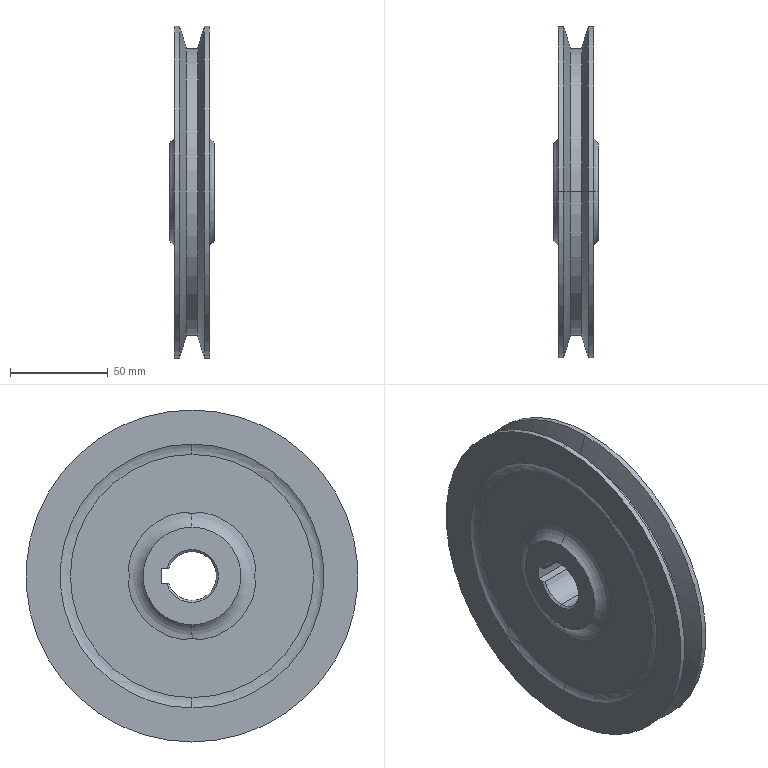Part | SolidWorks | features ICE 4, Cut 2, Chamfer 1, Fillet 1, RevCut 1, Revolution 1 | 1 solid | 46 faces | box 23 x 169.7 x 169.7 mm | volume 320640 mm3 | cylinder 19 | cone 10 | plane 9 | torus 8 | commonest cylinder face diameters 28.4 x10 169.7 x4 25 x3 146.8 x2
STEP:
#1=CARTESIAN_POINT('',(16.5,4.414,-32.703));
#2=VERTEX_POINT('',#1);
#3=CARTESIAN_POINT('',(16.55,0.,-32.));
#4=VERTEX_POINT('',#3);
#5=CARTESIAN_POINT('',(16.5,4.414,-32.703));
#6=CARTESIAN_POINT('',(16.5,3.701,-32.47));
#7=CARTESIAN_POINT('',(16.515,2.977,-32.296));
#8=CARTESIAN_POINT('',(16.534,1.874,-32.119));
#9=CARTESIAN_POINT('',(16.54,1.503,-32.075));
#10=CARTESIAN_POINT('',(16.548,0.7555,-32.015));
#11=CARTESIAN_POINT('',(16.55,0.3773,-32.));
#12=CARTESIAN_POINT('',(16.55,0.,-32.));
#13=B_SPLINE_CURVE_WITH_KNOTS('',3,(#5,#6,#7,#8,#9,#10,#11,#12),.UNSPECIFIED.,.F.,.F.,(4,2,2,4),(0.0008632,0.003097,0.004214,0.00533),.UNSPECIFIED.);
#14=EDGE_CURVE('',#2,#4,#13,.T.);
#15=ORIENTED_EDGE('',*,*,#14,.T.);
#16=CARTESIAN_POINT('',(16.5,0.,-32.));
#17=VERTEX_POINT('',#16);
#18=CARTESIAN_POINT('',(20.5,0.,-32.));
#19=DIRECTION('',(-1.,0.,0.));
#20=VECTOR('',#19,1000.);
#21=LINE('',#18,#20);
#22=EDGE_CURVE('',#4,#17,#21,.T.);
#23=ORIENTED_EDGE('',*,*,#22,.T.);
#24=CARTESIAN_POINT('',(16.5,0.,-46.2));
#25=DIRECTION('',(1.,0.,0.));
#26=DIRECTION('',(0.,0.,-1.));
#27=AXIS2_PLACEMENT_3D('',#24,#25,#26);
#28=CIRCLE('',#27,14.2);
#29=EDGE_CURVE('',#2,#17,#28,.T.);
#30=ORIENTED_EDGE('',*,*,#29,.F.);
#31=EDGE_LOOP('',(#15,#23,#30));
#32=FACE_OUTER_BOUND('',#31,.T.);
#33=CARTESIAN_POINT('',(20.5,0.,-46.2));
#34=DIRECTION('',(-1.,0.,0.));
#35=DIRECTION('',(0.,0.,1.));
#36=AXIS2_PLACEMENT_3D('',#33,#34,#35);
#37=CYLINDRICAL_SURFACE('',#36,14.2);
#38=ADVANCED_FACE('',(#32),#37,.F.);
#39=CARTESIAN_POINT('',(16.5,0.,62.132));
#40=VERTEX_POINT('',#39);
#41=CARTESIAN_POINT('',(16.5,0.,-62.132));
#42=VERTEX_POINT('',#41);
#43=CARTESIAN_POINT('',(16.5,0.,0.));
#44=DIRECTION('',(1.,0.,0.));
#45=DIRECTION('',(0.,0.,1.));
#46=AXIS2_PLACEMENT_3D('',#43,#44,#45);
#47=CIRCLE('',#46,62.132);
#48=EDGE_CURVE('',#40,#42,#47,.T.);
#49=ORIENTED_EDGE('',*,*,#48,.F.);
#50=CARTESIAN_POINT('',(18.,0.,67.4));
#51=VERTEX_POINT('',#50);
#52=CARTESIAN_POINT('',(26.5,0.,62.132));
#53=DIRECTION('',(0.,1.,0.));
#54=DIRECTION('',(0.,0.,1.));
#55=AXIS2_PLACEMENT_3D('',#52,#53,#54);
#56=CIRCLE('',#55,10.);
#57=EDGE_CURVE('',#40,#51,#56,.T.);
#58=ORIENTED_EDGE('',*,*,#57,.T.);
#59=CARTESIAN_POINT('',(18.,0.,-67.4));
#60=VERTEX_POINT('',#59);
#61=CARTESIAN_POINT('',(18.,0.,0.));
#62=DIRECTION('',(-1.,0.,0.));
#63=DIRECTION('',(0.,0.,1.));
#64=AXIS2_PLACEMENT_3D('',#61,#62,#63);
#65=CIRCLE('',#64,67.4);
#66=EDGE_CURVE('',#60,#51,#65,.T.);
#67=ORIENTED_EDGE('',*,*,#66,.F.);
#68=CARTESIAN_POINT('',(26.5,0.,-62.132));
#69=DIRECTION('',(0.,-1.,0.));
#70=DIRECTION('',(0.,0.,-1.));
#71=AXIS2_PLACEMENT_3D('',#68,#69,#70);
#72=CIRCLE('',#71,10.);
#73=EDGE_CURVE('',#42,#60,#72,.T.);
#74=ORIENTED_EDGE('',*,*,#73,.F.);
#75=EDGE_LOOP('',(#49,#58,#67,#74));
#76=FACE_OUTER_BOUND('',#75,.T.);
#77=CARTESIAN_POINT('',(26.5,0.,0.));
#78=DIRECTION('',(1.,0.,0.));
#79=DIRECTION('',(0.,0.,-1.));
#80=AXIS2_PLACEMENT_3D('',#77,#78,#79);
#81=TOROIDAL_SURFACE('',#80,62.132,10.);
#82=ADVANCED_FACE('',(#76),#81,.F.);
#83=CARTESIAN_POINT('',(1.5,0.,-62.132));
#84=VERTEX_POINT('',#83);
#85=CARTESIAN_POINT('',(1.5,0.,62.132));
#86=VERTEX_POINT('',#85);
#87=CARTESIAN_POINT('',(1.5,0.,0.));
#88=DIRECTION('',(-1.,0.,0.));
#89=DIRECTION('',(0.,0.,-1.));
#90=AXIS2_PLACEMENT_3D('',#87,#88,#89);
#91=CIRCLE('',#90,62.132);
#92=EDGE_CURVE('',#84,#86,#91,.T.);
#93=ORIENTED_EDGE('',*,*,#92,.F.);
#94=CARTESIAN_POINT('',(0.,0.,-67.4));
#95=VERTEX_POINT('',#94);
#96=CARTESIAN_POINT('',(-8.5,0.,-62.132));
#97=DIRECTION('',(0.,1.,0.));
#98=DIRECTION('',(0.,0.,1.));
#99=AXIS2_PLACEMENT_3D('',#96,#97,#98);
#100=CIRCLE('',#99,10.);
#101=EDGE_CURVE('',#84,#95,#100,.T.);
#102=ORIENTED_EDGE('',*,*,#101,.T.);
#103=CARTESIAN_POINT('',(0.,0.,67.4));
#104=VERTEX_POINT('',#103);
#105=CARTESIAN_POINT('',(0.,0.,0.));
#106=DIRECTION('',(-1.,0.,0.));
#107=DIRECTION('',(0.,0.,1.));
#108=AXIS2_PLACEMENT_3D('',#105,#106,#107);
#109=CIRCLE('',#108,67.4);
#110=EDGE_CURVE('',#95,#104,#109,.T.);
#111=ORIENTED_EDGE('',*,*,#110,.T.);
#112=CARTESIAN_POINT('',(-8.5,0.,62.132));
#113=DIRECTION('',(0.,-1.,0.));
#114=DIRECTION('',(0.,0.,-1.));
#115=AXIS2_PLACEMENT_3D('',#112,#113,#114);
#116=CIRCLE('',#115,10.);
#117=EDGE_CURVE('',#86,#104,#116,.T.);
#118=ORIENTED_EDGE('',*,*,#117,.F.);
#119=EDGE_LOOP('',(#93,#102,#111,#118));
#120=FACE_OUTER_BOUND('',#119,.T.);
#121=CARTESIAN_POINT('',(-8.5,0.,0.));
#122=DIRECTION('',(-1.,0.,0.));
#123=DIRECTION('',(0.,0.,1.));
#124=AXIS2_PLACEMENT_3D('',#121,#122,#123);
#125=TOROIDAL_SURFACE('',#124,62.132,10.);
#126=ADVANCED_FACE('',(#120),#125,.F.);
#127=CARTESIAN_POINT('',(19.5,0.,12.5));
#128=VERTEX_POINT('',#127);
#129=CARTESIAN_POINT('',(19.5,0.,-12.5));
#130=VERTEX_POINT('',#129);
#131=CARTESIAN_POINT('',(19.5,0.,0.));
#132=DIRECTION('',(1.,0.,0.));
#133=DIRECTION('',(0.,0.,1.));
#134=AXIS2_PLACEMENT_3D('',#131,#132,#133);
#135=CIRCLE('',#134,12.5);
#136=EDGE_CURVE('',#128,#130,#135,.T.);
#137=ORIENTED_EDGE('',*,*,#136,.F.);
#138=CARTESIAN_POINT('',(20.5,0.,13.5));
#139=VERTEX_POINT('',#138);
#140=CARTESIAN_POINT('',(20.5,0.,13.5));
#141=DIRECTION('',(0.7071,0.,0.7071));
#142=VECTOR('',#141,1000.);
#143=LINE('',#140,#142);
#144=EDGE_CURVE('',#128,#139,#143,.T.);
#145=ORIENTED_EDGE('',*,*,#144,.T.);
#146=CARTESIAN_POINT('',(20.5,0.,-13.5));
#147=VERTEX_POINT('',#146);
#148=CARTESIAN_POINT('',(20.5,0.,0.));
#149=DIRECTION('',(-1.,0.,0.));
#150=DIRECTION('',(0.,0.,1.));
#151=AXIS2_PLACEMENT_3D('',#148,#149,#150);
#152=CIRCLE('',#151,13.5);
#153=EDGE_CURVE('',#147,#139,#152,.T.);
#154=ORIENTED_EDGE('',*,*,#153,.F.);
#155=CARTESIAN_POINT('',(20.5,0.,-13.5));
#156=DIRECTION('',(0.7071,0.,-0.7071));
#157=VECTOR('',#156,1000.);
#158=LINE('',#155,#157);
#159=EDGE_CURVE('',#130,#147,#158,.T.);
#160=ORIENTED_EDGE('',*,*,#159,.F.);
#161=EDGE_LOOP('',(#137,#145,#154,#160));
#162=FACE_OUTER_BOUND('',#161,.T.);
#163=CARTESIAN_POINT('',(20.5,0.,0.));
#164=DIRECTION('',(1.,0.,0.));
#165=DIRECTION('',(0.,0.,-1.));
#166=AXIS2_PLACEMENT_3D('',#163,#164,#165);
#167=CONICAL_SURFACE('',#166,13.5,0.7854);
#168=ADVANCED_FACE('',(#162),#167,.F.);
#169=CARTESIAN_POINT('',(19.5,11.843,-4.));
#170=VERTEX_POINT('',#169);
#171=CARTESIAN_POINT('',(19.5,0.,0.));
#172=DIRECTION('',(1.,0.,0.));
#173=DIRECTION('',(0.,0.,1.));
#174=AXIS2_PLACEMENT_3D('',#171,#172,#173);
#175=CIRCLE('',#174,12.5);
#176=EDGE_CURVE('',#130,#170,#175,.T.);
#177=ORIENTED_EDGE('',*,*,#176,.F.);
#178=ORIENTED_EDGE('',*,*,#159,.T.);
#179=CARTESIAN_POINT('',(20.5,12.894,-4.));
#180=VERTEX_POINT('',#179);
#181=CARTESIAN_POINT('',(20.5,0.,0.));
#182=DIRECTION('',(-1.,0.,0.));
#183=DIRECTION('',(0.,0.,1.));
#184=AXIS2_PLACEMENT_3D('',#181,#182,#183);
#185=CIRCLE('',#184,13.5);
#186=EDGE_CURVE('',#180,#147,#185,.T.);
#187=ORIENTED_EDGE('',*,*,#186,.F.);
#188=CARTESIAN_POINT('',(19.5,11.843,-4.));
#189=CARTESIAN_POINT('',(19.833,12.194,-4.));
#190=CARTESIAN_POINT('',(20.166,12.544,-4.));
#191=CARTESIAN_POINT('',(20.5,12.894,-4.));
#192=B_SPLINE_CURVE_WITH_KNOTS('',3,(#188,#189,#190,#191),.UNSPECIFIED.,.F.,.F.,(4,4),(0.00346,0.004911),.UNSPECIFIED.);
#193=EDGE_CURVE('',#170,#180,#192,.T.);
#194=ORIENTED_EDGE('',*,*,#193,.F.);
#195=EDGE_LOOP('',(#177,#178,#187,#194));
#196=FACE_OUTER_BOUND('',#195,.T.);
#197=CARTESIAN_POINT('',(20.5,0.,0.));
#198=DIRECTION('',(1.,0.,0.));
#199=DIRECTION('',(0.,0.,-1.));
#200=AXIS2_PLACEMENT_3D('',#197,#198,#199);
#201=CONICAL_SURFACE('',#200,13.5,0.7854);
#202=ADVANCED_FACE('',(#196),#201,.F.);
#203=CARTESIAN_POINT('',(-1.5,0.,-12.5));
#204=VERTEX_POINT('',#203);
#205=CARTESIAN_POINT('',(-1.5,0.,12.5));
#206=VERTEX_POINT('',#205);
#207=CARTESIAN_POINT('',(-1.5,0.,0.));
#208=DIRECTION('',(-1.,0.,0.));
#209=DIRECTION('',(0.,0.,-1.));
#210=AXIS2_PLACEMENT_3D('',#207,#208,#209);
#211=CIRCLE('',#210,12.5);
#212=EDGE_CURVE('',#204,#206,#211,.T.);
#213=ORIENTED_EDGE('',*,*,#212,.F.);
#214=CARTESIAN_POINT('',(-2.5,0.,-13.5));
#215=VERTEX_POINT('',#214);
#216=CARTESIAN_POINT('',(-1.5,0.,-12.5));
#217=DIRECTION('',(-0.7071,0.,-0.7071));
#218=VECTOR('',#217,1000.);
#219=LINE('',#216,#218);
#220=EDGE_CURVE('',#204,#215,#219,.T.);
#221=ORIENTED_EDGE('',*,*,#220,.T.);
#222=CARTESIAN_POINT('',(-2.5,0.,13.5));
#223=VERTEX_POINT('',#222);
#224=CARTESIAN_POINT('',(-2.5,0.,0.));
#225=DIRECTION('',(1.,0.,0.));
#226=DIRECTION('',(0.,0.,-1.));
#227=AXIS2_PLACEMENT_3D('',#224,#225,#226);
#228=CIRCLE('',#227,13.5);
#229=EDGE_CURVE('',#223,#215,#228,.T.);
#230=ORIENTED_EDGE('',*,*,#229,.F.);
#231=CARTESIAN_POINT('',(-1.5,0.,12.5));
#232=DIRECTION('',(-0.7071,0.,0.7071));
#233=VECTOR('',#232,1000.);
#234=LINE('',#231,#233);
#235=EDGE_CURVE('',#206,#223,#234,.T.);
#236=ORIENTED_EDGE('',*,*,#235,.F.);
#237=EDGE_LOOP('',(#213,#221,#230,#236));
#238=FACE_OUTER_BOUND('',#237,.T.);
#239=CARTESIAN_POINT('',(-1.5,0.,0.));
#240=DIRECTION('',(-1.,0.,0.));
#241=DIRECTION('',(0.,0.,1.));
#242=AXIS2_PLACEMENT_3D('',#239,#240,#241);
#243=CONICAL_SURFACE('',#242,12.5,0.7854);
#244=ADVANCED_FACE('',(#238),#243,.F.);
#245=CARTESIAN_POINT('',(-1.5,11.843,4.));
#246=VERTEX_POINT('',#245);
#247=CARTESIAN_POINT('',(-1.5,0.,0.));
#248=DIRECTION('',(-1.,0.,0.));
#249=DIRECTION('',(0.,0.,-1.));
#250=AXIS2_PLACEMENT_3D('',#247,#248,#249);
#251=CIRCLE('',#250,12.5);
#252=EDGE_CURVE('',#206,#246,#251,.T.);
#253=ORIENTED_EDGE('',*,*,#252,.F.);
#254=ORIENTED_EDGE('',*,*,#235,.T.);
#255=CARTESIAN_POINT('',(-2.5,12.894,4.));
#256=VERTEX_POINT('',#255);
#257=CARTESIAN_POINT('',(-2.5,0.,0.));
#258=DIRECTION('',(1.,0.,0.));
#259=DIRECTION('',(0.,0.,-1.));
#260=AXIS2_PLACEMENT_3D('',#257,#258,#259);
#261=CIRCLE('',#260,13.5);
#262=EDGE_CURVE('',#256,#223,#261,.T.);
#263=ORIENTED_EDGE('',*,*,#262,.F.);
#264=CARTESIAN_POINT('',(-1.5,11.843,4.));
#265=CARTESIAN_POINT('',(-1.833,12.194,4.));
#266=CARTESIAN_POINT('',(-2.166,12.544,4.));
#267=CARTESIAN_POINT('',(-2.5,12.894,4.));
#268=B_SPLINE_CURVE_WITH_KNOTS('',3,(#264,#265,#266,#267),.UNSPECIFIED.,.F.,.F.,(4,4),(0.002815,0.004266),.UNSPECIFIED.);
#269=EDGE_CURVE('',#246,#256,#268,.T.);
#270=ORIENTED_EDGE('',*,*,#269,.F.);
#271=EDGE_LOOP('',(#253,#254,#263,#270));
#272=FACE_OUTER_BOUND('',#271,.T.);
#273=CARTESIAN_POINT('',(-1.5,0.,0.));
#274=DIRECTION('',(-1.,0.,0.));
#275=DIRECTION('',(0.,0.,1.));
#276=AXIS2_PLACEMENT_3D('',#273,#274,#275);
#277=CONICAL_SURFACE('',#276,12.5,0.7854);
#278=ADVANCED_FACE('',(#272),#277,.F.);
#279=CARTESIAN_POINT('',(6.16,0.,73.4));
#280=VERTEX_POINT('',#279);
#281=CARTESIAN_POINT('',(6.16,0.,-73.4));
#282=VERTEX_POINT('',#281);
#283=CARTESIAN_POINT('',(6.16,0.,0.));
#284=DIRECTION('',(-1.,0.,0.));
#285=DIRECTION('',(0.,0.,1.));
#286=AXIS2_PLACEMENT_3D('',#283,#284,#285);
#287=CIRCLE('',#286,73.4);
#288=EDGE_CURVE('',#280,#282,#287,.T.);
#289=ORIENTED_EDGE('',*,*,#288,.T.);
#290=CARTESIAN_POINT('',(2.659,0.,-84.85));
#291=VERTEX_POINT('',#290);
#292=CARTESIAN_POINT('',(2.659,0.,-84.85));
#293=DIRECTION('',(-0.2924,0.,-0.9563));
#294=VECTOR('',#293,1000.);
#295=LINE('',#292,#294);
#296=EDGE_CURVE('',#282,#291,#295,.T.);
#297=ORIENTED_EDGE('',*,*,#296,.T.);
#298=CARTESIAN_POINT('',(2.659,0.,84.85));
#299=VERTEX_POINT('',#298);
#300=CARTESIAN_POINT('',(2.659,0.,0.));
#301=DIRECTION('',(-1.,0.,0.));
#302=DIRECTION('',(0.,0.,1.));
#303=AXIS2_PLACEMENT_3D('',#300,#301,#302);
#304=CIRCLE('',#303,84.85);
#305=EDGE_CURVE('',#299,#291,#304,.T.);
#306=ORIENTED_EDGE('',*,*,#305,.F.);
#307=CARTESIAN_POINT('',(2.659,0.,84.85));
#308=DIRECTION('',(-0.2924,0.,0.9563));
#309=VECTOR('',#308,1000.);
#310=LINE('',#307,#309);
#311=EDGE_CURVE('',#280,#299,#310,.T.);
#312=ORIENTED_EDGE('',*,*,#311,.F.);
#313=EDGE_LOOP('',(#289,#297,#306,#312));
#314=FACE_OUTER_BOUND('',#313,.T.);
#315=CARTESIAN_POINT('',(2.659,0.,0.));
#316=DIRECTION('',(-1.,0.,0.));
#317=DIRECTION('',(0.,0.,1.));
#318=AXIS2_PLACEMENT_3D('',#315,#316,#317);
#319=CONICAL_SURFACE('',#318,84.85,1.274);
#320=ADVANCED_FACE('',(#314),#319,.T.);
#321=CARTESIAN_POINT('',(11.84,0.,73.4));
#322=VERTEX_POINT('',#321);
#323=CARTESIAN_POINT('',(11.84,0.,-73.4));
#324=VERTEX_POINT('',#323);
#325=CARTESIAN_POINT('',(11.84,0.,0.));
#326=DIRECTION('',(-1.,0.,0.));
#327=DIRECTION('',(0.,0.,1.));
#328=AXIS2_PLACEMENT_3D('',#325,#326,#327);
#329=CIRCLE('',#328,73.4);
#330=EDGE_CURVE('',#322,#324,#329,.T.);
#331=ORIENTED_EDGE('',*,*,#330,.F.);
#332=CARTESIAN_POINT('',(15.341,0.,84.85));
#333=VERTEX_POINT('',#332);
#334=CARTESIAN_POINT('',(11.84,0.,73.4));
#335=DIRECTION('',(0.2924,0.,0.9563));
#336=VECTOR('',#335,1000.);
#337=LINE('',#334,#336);
#338=EDGE_CURVE('',#322,#333,#337,.T.);
#339=ORIENTED_EDGE('',*,*,#338,.T.);
#340=CARTESIAN_POINT('',(15.341,0.,-84.85));
#341=VERTEX_POINT('',#340);
#342=CARTESIAN_POINT('',(15.341,0.,0.));
#343=DIRECTION('',(-1.,0.,0.));
#344=DIRECTION('',(0.,0.,1.));
#345=AXIS2_PLACEMENT_3D('',#342,#343,#344);
#346=CIRCLE('',#345,84.85);
#347=EDGE_CURVE('',#333,#341,#346,.T.);
#348=ORIENTED_EDGE('',*,*,#347,.T.);
#349=CARTESIAN_POINT('',(11.84,0.,-73.4));
#350=DIRECTION('',(0.2924,0.,-0.9563));
#351=VECTOR('',#350,1000.);
#352=LINE('',#349,#351);
#353=EDGE_CURVE('',#324,#341,#352,.T.);
#354=ORIENTED_EDGE('',*,*,#353,.F.);
#355=EDGE_LOOP('',(#331,#339,#348,#354));
#356=FACE_OUTER_BOUND('',#355,.T.);
#357=CARTESIAN_POINT('',(11.84,0.,0.));
#358=DIRECTION('',(1.,0.,0.));
#359=DIRECTION('',(0.,0.,-1.));
#360=AXIS2_PLACEMENT_3D('',#357,#358,#359);
#361=CONICAL_SURFACE('',#360,73.4,1.274);
#362=ADVANCED_FACE('',(#356),#361,.T.);
#363=ORIENTED_EDGE('',*,*,#330,.T.);
#364=CARTESIAN_POINT('',(0.,0.,-73.4));
#365=DIRECTION('',(-1.,0.,0.));
#366=VECTOR('',#365,1000.);
#367=LINE('',#364,#366);
#368=EDGE_CURVE('',#324,#282,#367,.T.);
#369=ORIENTED_EDGE('',*,*,#368,.T.);
#370=ORIENTED_EDGE('',*,*,#288,.F.);
#371=CARTESIAN_POINT('',(0.,0.,73.4));
#372=DIRECTION('',(-1.,0.,0.));
#373=VECTOR('',#372,1000.);
#374=LINE('',#371,#373);
#375=EDGE_CURVE('',#322,#280,#374,.T.);
#376=ORIENTED_EDGE('',*,*,#375,.F.);
#377=EDGE_LOOP('',(#363,#369,#370,#376));
#378=FACE_OUTER_BOUND('',#377,.T.);
#379=CARTESIAN_POINT('',(0.,0.,0.));
#380=DIRECTION('',(-1.,0.,0.));
#381=DIRECTION('',(0.,0.,1.));
#382=AXIS2_PLACEMENT_3D('',#379,#380,#381);
#383=CYLINDRICAL_SURFACE('',#382,73.4);
#384=ADVANCED_FACE('',(#378),#383,.T.);
#385=ORIENTED_EDGE('',*,*,#136,.T.);
#386=CARTESIAN_POINT('',(0.,0.,-12.5));
#387=DIRECTION('',(-1.,0.,0.));
#388=VECTOR('',#387,1000.);
#389=LINE('',#386,#388);
#390=EDGE_CURVE('',#130,#204,#389,.T.);
#391=ORIENTED_EDGE('',*,*,#390,.T.);
#392=ORIENTED_EDGE('',*,*,#212,.T.);
#393=CARTESIAN_POINT('',(0.,0.,12.5));
#394=DIRECTION('',(-1.,0.,0.));
#395=VECTOR('',#394,1000.);
#396=LINE('',#393,#395);
#397=EDGE_CURVE('',#128,#206,#396,.T.);
#398=ORIENTED_EDGE('',*,*,#397,.F.);
#399=EDGE_LOOP('',(#385,#391,#392,#398));
#400=FACE_OUTER_BOUND('',#399,.T.);
#401=CARTESIAN_POINT('',(0.,0.,0.));
#402=DIRECTION('',(-1.,0.,0.));
#403=DIRECTION('',(0.,0.,1.));
#404=AXIS2_PLACEMENT_3D('',#401,#402,#403);
#405=CYLINDRICAL_SURFACE('',#404,12.5);
#406=ADVANCED_FACE('',(#400),#405,.F.);
#407=CARTESIAN_POINT('',(19.5,11.843,4.));
#408=VERTEX_POINT('',#407);
#409=CARTESIAN_POINT('',(19.5,0.,0.));
#410=DIRECTION('',(1.,0.,0.));
#411=DIRECTION('',(0.,0.,1.));
#412=AXIS2_PLACEMENT_3D('',#409,#410,#411);
#413=CIRCLE('',#412,12.5);
#414=EDGE_CURVE('',#408,#128,#413,.T.);
#415=ORIENTED_EDGE('',*,*,#414,.T.);
#416=ORIENTED_EDGE('',*,*,#397,.T.);
#417=ORIENTED_EDGE('',*,*,#252,.T.);
#418=CARTESIAN_POINT('',(20.5,11.843,4.));
#419=DIRECTION('',(-1.,0.,0.));
#420=VECTOR('',#419,1000.);
#421=LINE('',#418,#420);
#422=EDGE_CURVE('',#408,#246,#421,.T.);
#423=ORIENTED_EDGE('',*,*,#422,.F.);
#424=EDGE_LOOP('',(#415,#416,#417,#423));
#425=FACE_OUTER_BOUND('',#424,.T.);
#426=CARTESIAN_POINT('',(0.,0.,0.));
#427=DIRECTION('',(-1.,0.,0.));
#428=DIRECTION('',(0.,0.,1.));
#429=AXIS2_PLACEMENT_3D('',#426,#427,#428);
#430=CYLINDRICAL_SURFACE('',#429,12.5);
#431=ADVANCED_FACE('',(#425),#430,.F.);
#432=ORIENTED_EDGE('',*,*,#305,.T.);
#433=CARTESIAN_POINT('',(0.,0.,-84.85));
#434=VERTEX_POINT('',#433);
#435=CARTESIAN_POINT('',(0.,0.,-84.85));
#436=DIRECTION('',(-1.,0.,0.));
#437=VECTOR('',#436,1000.);
#438=LINE('',#435,#437);
#439=EDGE_CURVE('',#291,#434,#438,.T.);
#440=ORIENTED_EDGE('',*,*,#439,.T.);
#441=CARTESIAN_POINT('',(0.,0.,84.85));
#442=VERTEX_POINT('',#441);
#443=CARTESIAN_POINT('',(0.,0.,0.));
#444=DIRECTION('',(-1.,0.,0.));
#445=DIRECTION('',(0.,0.,1.));
#446=AXIS2_PLACEMENT_3D('',#443,#444,#445);
#447=CIRCLE('',#446,84.85);
#448=EDGE_CURVE('',#442,#434,#447,.T.);
#449=ORIENTED_EDGE('',*,*,#448,.F.);
#450=CARTESIAN_POINT('',(0.,0.,84.85));
#451=DIRECTION('',(-1.,0.,0.));
#452=VECTOR('',#451,1000.);
#453=LINE('',#450,#452);
#454=EDGE_CURVE('',#299,#442,#453,.T.);
#455=ORIENTED_EDGE('',*,*,#454,.F.);
#456=EDGE_LOOP('',(#432,#440,#449,#455));
#457=FACE_OUTER_BOUND('',#456,.T.);
#458=CARTESIAN_POINT('',(0.,0.,0.));
#459=DIRECTION('',(-1.,0.,0.));
#460=DIRECTION('',(0.,0.,1.));
#461=AXIS2_PLACEMENT_3D('',#458,#459,#460);
#462=CYLINDRICAL_SURFACE('',#461,84.85);
#463=ADVANCED_FACE('',(#457),#462,.T.);
#464=CARTESIAN_POINT('',(18.,0.,84.85));
#465=VERTEX_POINT('',#464);
#466=CARTESIAN_POINT('',(18.,0.,-84.85));
#467=VERTEX_POINT('',#466);
#468=CARTESIAN_POINT('',(18.,0.,0.));
#469=DIRECTION('',(-1.,0.,0.));
#470=DIRECTION('',(0.,0.,1.));
#471=AXIS2_PLACEMENT_3D('',#468,#469,#470);
#472=CIRCLE('',#471,84.85);
#473=EDGE_CURVE('',#465,#467,#472,.T.);
#474=ORIENTED_EDGE('',*,*,#473,.T.);
#475=CARTESIAN_POINT('',(0.,0.,-84.85));
#476=DIRECTION('',(-1.,0.,0.));
#477=VECTOR('',#476,1000.);
#478=LINE('',#475,#477);
#479=EDGE_CURVE('',#467,#341,#478,.T.);
#480=ORIENTED_EDGE('',*,*,#479,.T.);
#481=ORIENTED_EDGE('',*,*,#347,.F.);
#482=CARTESIAN_POINT('',(0.,0.,84.85));
#483=DIRECTION('',(-1.,0.,0.));
#484=VECTOR('',#483,1000.);
#485=LINE('',#482,#484);
#486=EDGE_CURVE('',#465,#333,#485,.T.);
#487=ORIENTED_EDGE('',*,*,#486,.F.);
#488=EDGE_LOOP('',(#474,#480,#481,#487));
#489=FACE_OUTER_BOUND('',#488,.T.);
#490=CARTESIAN_POINT('',(0.,0.,0.));
#491=DIRECTION('',(-1.,0.,0.));
#492=DIRECTION('',(0.,0.,1.));
#493=AXIS2_PLACEMENT_3D('',#490,#491,#492);
#494=CYLINDRICAL_SURFACE('',#493,84.85);
#495=ADVANCED_FACE('',(#489),#494,.T.);
#496=CARTESIAN_POINT('',(16.5,-4.414,-32.703));
#497=VERTEX_POINT('',#496);
#498=CARTESIAN_POINT('',(16.55,0.,-32.));
#499=CARTESIAN_POINT('',(16.55,-0.7535,-32.));
#500=CARTESIAN_POINT('',(16.54,-1.498,-32.06));
#501=CARTESIAN_POINT('',(16.515,-2.969,-32.294));
#502=CARTESIAN_POINT('',(16.5,-3.696,-32.469));
#503=CARTESIAN_POINT('',(16.5,-4.414,-32.703));
#504=B_SPLINE_CURVE_WITH_KNOTS('',3,(#498,#499,#500,#501,#502,#503),.UNSPECIFIED.,.F.,.F.,(4,2,4),(0.00533,0.007561,0.009791),.UNSPECIFIED.);
#505=EDGE_CURVE('',#4,#497,#504,.T.);
#506=ORIENTED_EDGE('',*,*,#505,.F.);
#507=CARTESIAN_POINT('',(20.5,0.,-25.));
#508=VERTEX_POINT('',#507);
#509=CARTESIAN_POINT('',(26.5,0.,-33.));
#510=DIRECTION('',(0.,1.,0.));
#511=DIRECTION('',(0.,0.,1.));
#512=AXIS2_PLACEMENT_3D('',#509,#510,#511);
#513=CIRCLE('',#512,10.);
#514=EDGE_CURVE('',#4,#508,#513,.T.);
#515=ORIENTED_EDGE('',*,*,#514,.T.);
#516=CARTESIAN_POINT('',(20.5,0.,25.));
#517=VERTEX_POINT('',#516);
#518=CARTESIAN_POINT('',(20.5,0.,0.));
#519=DIRECTION('',(-1.,0.,0.));
#520=DIRECTION('',(0.,0.,1.));
#521=AXIS2_PLACEMENT_3D('',#518,#519,#520);
#522=CIRCLE('',#521,25.);
#523=EDGE_CURVE('',#508,#517,#522,.T.);
#524=ORIENTED_EDGE('',*,*,#523,.T.);
#525=CARTESIAN_POINT('',(16.55,0.,32.));
#526=VERTEX_POINT('',#525);
#527=CARTESIAN_POINT('',(26.5,0.,33.));
#528=DIRECTION('',(0.,-1.,0.));
#529=DIRECTION('',(0.,0.,-1.));
#530=AXIS2_PLACEMENT_3D('',#527,#528,#529);
#531=CIRCLE('',#530,10.);
#532=EDGE_CURVE('',#526,#517,#531,.T.);
#533=ORIENTED_EDGE('',*,*,#532,.F.);
#534=CARTESIAN_POINT('',(16.5,-4.414,32.703));
#535=VERTEX_POINT('',#534);
#536=CARTESIAN_POINT('',(16.5,-4.414,32.703));
#537=CARTESIAN_POINT('',(16.5,-3.701,32.47));
#538=CARTESIAN_POINT('',(16.515,-2.977,32.296));
#539=CARTESIAN_POINT('',(16.534,-1.874,32.119));
#540=CARTESIAN_POINT('',(16.54,-1.503,32.075));
#541=CARTESIAN_POINT('',(16.548,-0.7555,32.015));
#542=CARTESIAN_POINT('',(16.55,-0.3773,32.));
#543=CARTESIAN_POINT('',(16.55,0.,32.));
#544=B_SPLINE_CURVE_WITH_KNOTS('',3,(#536,#537,#538,#539,#540,#541,#542,#543),.UNSPECIFIED.,.F.,.F.,(4,2,2,4),(0.0008632,0.003097,0.004214,0.00533),.UNSPECIFIED.);
#545=EDGE_CURVE('',#535,#526,#544,.T.);
#546=ORIENTED_EDGE('',*,*,#545,.F.);
#547=CARTESIAN_POINT('',(16.5,-32.703,4.414));
#548=VERTEX_POINT('',#547);
#549=CARTESIAN_POINT('',(16.5,0.,0.));
#550=DIRECTION('',(-1.,0.,0.));
#551=DIRECTION('',(0.,0.,1.));
#552=AXIS2_PLACEMENT_3D('',#549,#550,#551);
#553=CIRCLE('',#552,33.);
#554=EDGE_CURVE('',#548,#535,#553,.T.);
#555=ORIENTED_EDGE('',*,*,#554,.F.);
#556=CARTESIAN_POINT('',(16.5,-32.703,-4.414));
#557=VERTEX_POINT('',#556);
#558=CARTESIAN_POINT('',(16.5,-32.703,-4.414));
#559=CARTESIAN_POINT('',(16.5,-32.471,-3.702));
#560=CARTESIAN_POINT('',(16.515,-32.296,-2.978));
#561=CARTESIAN_POINT('',(16.534,-32.119,-1.876));
#562=CARTESIAN_POINT('',(16.54,-32.075,-1.505));
#563=CARTESIAN_POINT('',(16.548,-32.015,-0.7584));
#564=CARTESIAN_POINT('',(16.55,-32.,-0.3805));
#565=CARTESIAN_POINT('',(16.55,-32.,0.7506));
#566=CARTESIAN_POINT('',(16.54,-32.059,1.496));
#567=CARTESIAN_POINT('',(16.515,-32.294,2.968));
#568=CARTESIAN_POINT('',(16.5,-32.468,3.695));
#569=CARTESIAN_POINT('',(16.5,-32.703,4.414));
#570=B_SPLINE_CURVE_WITH_KNOTS('',3,(#558,#559,#560,#561,#562,#563,#564,#565,#566,#567,#568,#569),.UNSPECIFIED.,.F.,.F.,(4,2,2,2,2,4),(0.0008632,0.003095,0.004211,0.005327,0.007559,0.009791),.UNSPECIFIED.);
#571=EDGE_CURVE('',#557,#548,#570,.T.);
#572=ORIENTED_EDGE('',*,*,#571,.F.);
#573=CARTESIAN_POINT('',(16.5,0.,0.));
#574=DIRECTION('',(-1.,0.,0.));
#575=DIRECTION('',(0.,0.,1.));
#576=AXIS2_PLACEMENT_3D('',#573,#574,#575);
#577=CIRCLE('',#576,33.);
#578=EDGE_CURVE('',#497,#557,#577,.T.);
#579=ORIENTED_EDGE('',*,*,#578,.F.);
#580=EDGE_LOOP('',(#506,#515,#524,#533,#546,#555,#572,#579));
#581=FACE_OUTER_BOUND('',#580,.T.);
#582=CARTESIAN_POINT('',(26.5,0.,0.));
#583=DIRECTION('',(-1.,0.,0.));
#584=DIRECTION('',(0.,0.,1.));
#585=AXIS2_PLACEMENT_3D('',#582,#583,#584);
#586=TOROIDAL_SURFACE('',#585,33.,10.);
#587=ADVANCED_FACE('',(#581),#586,.F.);
#588=CARTESIAN_POINT('',(1.45,0.,32.));
#589=VERTEX_POINT('',#588);
#590=CARTESIAN_POINT('',(1.5,-4.414,32.703));
#591=VERTEX_POINT('',#590);
#592=CARTESIAN_POINT('',(1.45,0.,32.));
#593=CARTESIAN_POINT('',(1.45,-0.7535,32.));
#594=CARTESIAN_POINT('',(1.46,-1.498,32.06));
#595=CARTESIAN_POINT('',(1.485,-2.969,32.294));
#596=CARTESIAN_POINT('',(1.5,-3.696,32.469));
#597=CARTESIAN_POINT('',(1.5,-4.414,32.703));
#598=B_SPLINE_CURVE_WITH_KNOTS('',3,(#592,#593,#594,#595,#596,#597),.UNSPECIFIED.,.F.,.F.,(4,2,4),(0.00533,0.007561,0.009791),.UNSPECIFIED.);
#599=EDGE_CURVE('',#589,#591,#598,.T.);
#600=ORIENTED_EDGE('',*,*,#599,.F.);
#601=CARTESIAN_POINT('',(-2.5,0.,25.));
#602=VERTEX_POINT('',#601);
#603=CARTESIAN_POINT('',(-8.5,0.,33.));
#604=DIRECTION('',(0.,1.,0.));
#605=DIRECTION('',(0.,0.,1.));
#606=AXIS2_PLACEMENT_3D('',#603,#604,#605);
#607=CIRCLE('',#606,10.);
#608=EDGE_CURVE('',#589,#602,#607,.T.);
#609=ORIENTED_EDGE('',*,*,#608,.T.);
#610=CARTESIAN_POINT('',(-2.5,0.,-25.));
#611=VERTEX_POINT('',#610);
#612=CARTESIAN_POINT('',(-2.5,0.,0.));
#613=DIRECTION('',(-1.,0.,0.));
#614=DIRECTION('',(0.,0.,1.));
#615=AXIS2_PLACEMENT_3D('',#612,#613,#614);
#616=CIRCLE('',#615,25.);
#617=EDGE_CURVE('',#611,#602,#616,.T.);
#618=ORIENTED_EDGE('',*,*,#617,.F.);
#619=CARTESIAN_POINT('',(1.45,0.,-32.));
#620=VERTEX_POINT('',#619);
#621=CARTESIAN_POINT('',(-8.5,0.,-33.));
#622=DIRECTION('',(0.,-1.,0.));
#623=DIRECTION('',(0.,0.,-1.));
#624=AXIS2_PLACEMENT_3D('',#621,#622,#623);
#625=CIRCLE('',#624,10.);
#626=EDGE_CURVE('',#620,#611,#625,.T.);
#627=ORIENTED_EDGE('',*,*,#626,.F.);
#628=CARTESIAN_POINT('',(1.5,-4.414,-32.703));
#629=VERTEX_POINT('',#628);
#630=CARTESIAN_POINT('',(1.5,-4.414,-32.703));
#631=CARTESIAN_POINT('',(1.5,-3.701,-32.47));
#632=CARTESIAN_POINT('',(1.485,-2.977,-32.296));
#633=CARTESIAN_POINT('',(1.466,-1.874,-32.119));
#634=CARTESIAN_POINT('',(1.46,-1.503,-32.075));
#635=CARTESIAN_POINT('',(1.452,-0.7555,-32.015));
#636=CARTESIAN_POINT('',(1.45,-0.3773,-32.));
#637=CARTESIAN_POINT('',(1.45,0.,-32.));
#638=B_SPLINE_CURVE_WITH_KNOTS('',3,(#630,#631,#632,#633,#634,#635,#636,#637),.UNSPECIFIED.,.F.,.F.,(4,2,2,4),(0.0008632,0.003097,0.004214,0.00533),.UNSPECIFIED.);
#639=EDGE_CURVE('',#629,#620,#638,.T.);
#640=ORIENTED_EDGE('',*,*,#639,.F.);
#641=CARTESIAN_POINT('',(1.5,-32.703,-4.414));
#642=VERTEX_POINT('',#641);
#643=CARTESIAN_POINT('',(1.5,0.,0.));
#644=DIRECTION('',(1.,0.,0.));
#645=DIRECTION('',(0.,0.,-1.));
#646=AXIS2_PLACEMENT_3D('',#643,#644,#645);
#647=CIRCLE('',#646,33.);
#648=EDGE_CURVE('',#642,#629,#647,.T.);
#649=ORIENTED_EDGE('',*,*,#648,.F.);
#650=CARTESIAN_POINT('',(1.5,-32.703,4.414));
#651=VERTEX_POINT('',#650);
#652=CARTESIAN_POINT('',(1.5,-32.703,4.414));
#653=CARTESIAN_POINT('',(1.5,-32.471,3.702));
#654=CARTESIAN_POINT('',(1.485,-32.296,2.978));
#655=CARTESIAN_POINT('',(1.466,-32.119,1.876));
#656=CARTESIAN_POINT('',(1.46,-32.075,1.505));
#657=CARTESIAN_POINT('',(1.452,-32.015,0.7584));
#658=CARTESIAN_POINT('',(1.45,-32.,0.3805));
#659=CARTESIAN_POINT('',(1.45,-32.,-0.7506));
#660=CARTESIAN_POINT('',(1.46,-32.059,-1.496));
#661=CARTESIAN_POINT('',(1.485,-32.294,-2.968));
#662=CARTESIAN_POINT('',(1.5,-32.468,-3.695));
#663=CARTESIAN_POINT('',(1.5,-32.703,-4.414));
#664=B_SPLINE_CURVE_WITH_KNOTS('',3,(#652,#653,#654,#655,#656,#657,#658,#659,#660,#661,#662,#663),.UNSPECIFIED.,.F.,.F.,(4,2,2,2,2,4),(0.0008632,0.003095,0.004211,0.005327,0.007559,0.009791),.UNSPECIFIED.);
#665=EDGE_CURVE('',#651,#642,#664,.T.);
#666=ORIENTED_EDGE('',*,*,#665,.F.);
#667=CARTESIAN_POINT('',(1.5,0.,0.));
#668=DIRECTION('',(1.,0.,0.));
#669=DIRECTION('',(0.,0.,-1.));
#670=AXIS2_PLACEMENT_3D('',#667,#668,#669);
#671=CIRCLE('',#670,33.);
#672=EDGE_CURVE('',#591,#651,#671,.T.);
#673=ORIENTED_EDGE('',*,*,#672,.F.);
#674=EDGE_LOOP('',(#600,#609,#618,#627,#640,#649,#666,#673));
#675=FACE_OUTER_BOUND('',#674,.T.);
#676=CARTESIAN_POINT('',(-8.5,0.,0.));
#677=DIRECTION('',(1.,0.,0.));
#678=DIRECTION('',(0.,0.,-1.));
#679=AXIS2_PLACEMENT_3D('',#676,#677,#678);
#680=TOROIDAL_SURFACE('',#679,33.,10.);
#681=ADVANCED_FACE('',(#675),#680,.F.);
#682=CARTESIAN_POINT('',(1.5,4.414,-32.703));
#683=VERTEX_POINT('',#682);
#684=CARTESIAN_POINT('',(1.5,0.,-32.));
#685=VERTEX_POINT('',#684);
#686=CARTESIAN_POINT('',(1.5,0.,-46.2));
#687=DIRECTION('',(1.,0.,0.));
#688=DIRECTION('',(0.,0.,-1.));
#689=AXIS2_PLACEMENT_3D('',#686,#687,#688);
#690=CIRCLE('',#689,14.2);
#691=EDGE_CURVE('',#683,#685,#690,.T.);
#692=ORIENTED_EDGE('',*,*,#691,.T.);
#693=CARTESIAN_POINT('',(20.5,0.,-32.));
#694=DIRECTION('',(-1.,0.,0.));
#695=VECTOR('',#694,1000.);
#696=LINE('',#693,#695);
#697=EDGE_CURVE('',#685,#620,#696,.T.);
#698=ORIENTED_EDGE('',*,*,#697,.T.);
#699=CARTESIAN_POINT('',(1.45,0.,-32.));
#700=CARTESIAN_POINT('',(1.45,0.7535,-32.));
#701=CARTESIAN_POINT('',(1.46,1.498,-32.06));
#702=CARTESIAN_POINT('',(1.485,2.969,-32.294));
#703=CARTESIAN_POINT('',(1.5,3.696,-32.469));
#704=CARTESIAN_POINT('',(1.5,4.414,-32.703));
#705=B_SPLINE_CURVE_WITH_KNOTS('',3,(#699,#700,#701,#702,#703,#704),.UNSPECIFIED.,.F.,.F.,(4,2,4),(0.00533,0.007561,0.009791),.UNSPECIFIED.);
#706=EDGE_CURVE('',#620,#683,#705,.T.);
#707=ORIENTED_EDGE('',*,*,#706,.T.);
#708=EDGE_LOOP('',(#692,#698,#707));
#709=FACE_OUTER_BOUND('',#708,.T.);
#710=CARTESIAN_POINT('',(20.5,0.,-46.2));
#711=DIRECTION('',(-1.,0.,0.));
#712=DIRECTION('',(0.,0.,1.));
#713=AXIS2_PLACEMENT_3D('',#710,#711,#712);
#714=CYLINDRICAL_SURFACE('',#713,14.2);
#715=ADVANCED_FACE('',(#709),#714,.F.);
#716=ORIENTED_EDGE('',*,*,#665,.T.);
#717=CARTESIAN_POINT('',(1.5,-46.2,0.));
#718=DIRECTION('',(1.,0.,0.));
#719=DIRECTION('',(0.,0.,-1.));
#720=AXIS2_PLACEMENT_3D('',#717,#718,#719);
#721=CIRCLE('',#720,14.2);
#722=EDGE_CURVE('',#642,#651,#721,.T.);
#723=ORIENTED_EDGE('',*,*,#722,.T.);
#724=EDGE_LOOP('',(#716,#723));
#725=FACE_OUTER_BOUND('',#724,.T.);
#726=CARTESIAN_POINT('',(20.5,-46.2,0.));
#727=DIRECTION('',(-1.,0.,0.));
#728=DIRECTION('',(0.,0.,1.));
#729=AXIS2_PLACEMENT_3D('',#726,#727,#728);
#730=CYLINDRICAL_SURFACE('',#729,14.2);
#731=ADVANCED_FACE('',(#725),#730,.F.);
#732=ORIENTED_EDGE('',*,*,#697,.F.);
#733=CARTESIAN_POINT('',(1.5,0.,-46.2));
#734=DIRECTION('',(1.,0.,0.));
#735=DIRECTION('',(0.,0.,-1.));
#736=AXIS2_PLACEMENT_3D('',#733,#734,#735);
#737=CIRCLE('',#736,14.2);
#738=EDGE_CURVE('',#685,#629,#737,.T.);
#739=ORIENTED_EDGE('',*,*,#738,.T.);
#740=ORIENTED_EDGE('',*,*,#639,.T.);
#741=EDGE_LOOP('',(#732,#739,#740));
#742=FACE_OUTER_BOUND('',#741,.T.);
#743=CARTESIAN_POINT('',(20.5,0.,-46.2));
#744=DIRECTION('',(-1.,0.,0.));
#745=DIRECTION('',(0.,0.,1.));
#746=AXIS2_PLACEMENT_3D('',#743,#744,#745);
#747=CYLINDRICAL_SURFACE('',#746,14.2);
#748=ADVANCED_FACE('',(#742),#747,.F.);
#749=CARTESIAN_POINT('',(1.5,32.703,-4.414));
#750=VERTEX_POINT('',#749);
#751=CARTESIAN_POINT('',(1.5,32.703,4.414));
#752=VERTEX_POINT('',#751);
#753=CARTESIAN_POINT('',(1.5,32.703,-4.414));
#754=CARTESIAN_POINT('',(1.5,32.471,-3.702));
#755=CARTESIAN_POINT('',(1.485,32.296,-2.978));
#756=CARTESIAN_POINT('',(1.466,32.119,-1.876));
#757=CARTESIAN_POINT('',(1.46,32.075,-1.505));
#758=CARTESIAN_POINT('',(1.452,32.015,-0.7584));
#759=CARTESIAN_POINT('',(1.45,32.,-0.3805));
#760=CARTESIAN_POINT('',(1.45,32.,0.7506));
#761=CARTESIAN_POINT('',(1.46,32.059,1.496));
#762=CARTESIAN_POINT('',(1.485,32.294,2.968));
#763=CARTESIAN_POINT('',(1.5,32.468,3.695));
#764=CARTESIAN_POINT('',(1.5,32.703,4.414));
#765=B_SPLINE_CURVE_WITH_KNOTS('',3,(#753,#754,#755,#756,#757,#758,#759,#760,#761,#762,#763,#764),.UNSPECIFIED.,.F.,.F.,(4,2,2,2,2,4),(0.0008632,0.003095,0.004211,0.005327,0.007559,0.009791),.UNSPECIFIED.);
#766=EDGE_CURVE('',#750,#752,#765,.T.);
#767=ORIENTED_EDGE('',*,*,#766,.T.);
#768=CARTESIAN_POINT('',(1.5,46.2,0.));
#769=DIRECTION('',(1.,0.,0.));
#770=DIRECTION('',(0.,0.,-1.));
#771=AXIS2_PLACEMENT_3D('',#768,#769,#770);
#772=CIRCLE('',#771,14.2);
#773=EDGE_CURVE('',#752,#750,#772,.T.);
#774=ORIENTED_EDGE('',*,*,#773,.T.);
#775=EDGE_LOOP('',(#767,#774));
#776=FACE_OUTER_BOUND('',#775,.T.);
#777=CARTESIAN_POINT('',(20.5,46.2,0.));
#778=DIRECTION('',(-1.,0.,0.));
#779=DIRECTION('',(0.,0.,1.));
#780=AXIS2_PLACEMENT_3D('',#777,#778,#779);
#781=CYLINDRICAL_SURFACE('',#780,14.2);
#782=ADVANCED_FACE('',(#776),#781,.F.);
#783=CARTESIAN_POINT('',(1.5,4.414,32.703));
#784=VERTEX_POINT('',#783);
#785=CARTESIAN_POINT('',(1.5,4.414,32.703));
#786=CARTESIAN_POINT('',(1.5,3.701,32.47));
#787=CARTESIAN_POINT('',(1.485,2.977,32.296));
#788=CARTESIAN_POINT('',(1.466,1.874,32.119));
#789=CARTESIAN_POINT('',(1.46,1.503,32.075));
#790=CARTESIAN_POINT('',(1.452,0.7555,32.015));
#791=CARTESIAN_POINT('',(1.45,0.3773,32.));
#792=CARTESIAN_POINT('',(1.45,0.,32.));
#793=B_SPLINE_CURVE_WITH_KNOTS('',3,(#785,#786,#787,#788,#789,#790,#791,#792),.UNSPECIFIED.,.F.,.F.,(4,2,2,4),(0.0008632,0.003097,0.004214,0.00533),.UNSPECIFIED.);
#794=EDGE_CURVE('',#784,#589,#793,.T.);
#795=ORIENTED_EDGE('',*,*,#794,.T.);
#796=ORIENTED_EDGE('',*,*,#599,.T.);
#797=CARTESIAN_POINT('',(1.5,0.,46.2));
#798=DIRECTION('',(1.,0.,0.));
#799=DIRECTION('',(0.,0.,-1.));
#800=AXIS2_PLACEMENT_3D('',#797,#798,#799);
#801=CIRCLE('',#800,14.2);
#802=EDGE_CURVE('',#591,#784,#801,.T.);
#803=ORIENTED_EDGE('',*,*,#802,.T.);
#804=EDGE_LOOP('',(#795,#796,#803));
#805=FACE_OUTER_BOUND('',#804,.T.);
#806=CARTESIAN_POINT('',(20.5,0.,46.2));
#807=DIRECTION('',(-1.,0.,0.));
#808=DIRECTION('',(0.,0.,1.));
#809=AXIS2_PLACEMENT_3D('',#806,#807,#808);
#810=CYLINDRICAL_SURFACE('',#809,14.2);
#811=ADVANCED_FACE('',(#805),#810,.F.);
#812=CARTESIAN_POINT('',(1.5,0.,0.));
#813=DIRECTION('',(-1.,0.,0.));
#814=DIRECTION('',(0.,0.,-1.));
#815=AXIS2_PLACEMENT_3D('',#812,#813,#814);
#816=CIRCLE('',#815,62.132);
#817=EDGE_CURVE('',#86,#84,#816,.T.);
#818=ORIENTED_EDGE('',*,*,#817,.T.);
#819=ORIENTED_EDGE('',*,*,#92,.T.);
#820=EDGE_LOOP('',(#818,#819));
#821=FACE_OUTER_BOUND('',#820,.T.);
#822=CARTESIAN_POINT('',(1.5,0.,0.));
#823=DIRECTION('',(1.,0.,0.));
#824=DIRECTION('',(0.,0.,-1.));
#825=AXIS2_PLACEMENT_3D('',#822,#823,#824);
#826=CIRCLE('',#825,33.);
#827=EDGE_CURVE('',#752,#784,#826,.T.);
#828=ORIENTED_EDGE('',*,*,#827,.T.);
#829=ORIENTED_EDGE('',*,*,#802,.F.);
#830=ORIENTED_EDGE('',*,*,#672,.T.);
#831=ORIENTED_EDGE('',*,*,#722,.F.);
#832=ORIENTED_EDGE('',*,*,#648,.T.);
#833=ORIENTED_EDGE('',*,*,#738,.F.);
#834=ORIENTED_EDGE('',*,*,#691,.F.);
#835=CARTESIAN_POINT('',(1.5,0.,0.));
#836=DIRECTION('',(1.,0.,0.));
#837=DIRECTION('',(0.,0.,-1.));
#838=AXIS2_PLACEMENT_3D('',#835,#836,#837);
#839=CIRCLE('',#838,33.);
#840=EDGE_CURVE('',#683,#750,#839,.T.);
#841=ORIENTED_EDGE('',*,*,#840,.T.);
#842=ORIENTED_EDGE('',*,*,#773,.F.);
#843=EDGE_LOOP('',(#828,#829,#830,#831,#832,#833,#834,#841,#842));
#844=FACE_BOUND('',#843,.T.);
#845=CARTESIAN_POINT('',(1.5,25.35,0.));
#846=DIRECTION('',(1.,0.,0.));
#847=DIRECTION('',(0.,0.,-1.));
#848=AXIS2_PLACEMENT_3D('',#845,#846,#847);
#849=PLANE('',#848);
#850=ADVANCED_FACE('',(#821,#844),#849,.F.);
#851=CARTESIAN_POINT('',(16.5,0.,0.));
#852=DIRECTION('',(1.,0.,0.));
#853=DIRECTION('',(0.,0.,1.));
#854=AXIS2_PLACEMENT_3D('',#851,#852,#853);
#855=CIRCLE('',#854,62.132);
#856=EDGE_CURVE('',#42,#40,#855,.T.);
#857=ORIENTED_EDGE('',*,*,#856,.T.);
#858=ORIENTED_EDGE('',*,*,#48,.T.);
#859=EDGE_LOOP('',(#857,#858));
#860=FACE_OUTER_BOUND('',#859,.T.);
#861=ORIENTED_EDGE('',*,*,#554,.T.);
#862=CARTESIAN_POINT('',(16.5,4.414,32.703));
#863=VERTEX_POINT('',#862);
#864=CARTESIAN_POINT('',(16.5,0.,46.2));
#865=DIRECTION('',(1.,0.,0.));
#866=DIRECTION('',(0.,0.,-1.));
#867=AXIS2_PLACEMENT_3D('',#864,#865,#866);
#868=CIRCLE('',#867,14.2);
#869=EDGE_CURVE('',#535,#863,#868,.T.);
#870=ORIENTED_EDGE('',*,*,#869,.T.);
#871=CARTESIAN_POINT('',(16.5,32.703,4.414));
#872=VERTEX_POINT('',#871);
#873=CARTESIAN_POINT('',(16.5,0.,0.));
#874=DIRECTION('',(-1.,0.,0.));
#875=DIRECTION('',(0.,0.,1.));
#876=AXIS2_PLACEMENT_3D('',#873,#874,#875);
#877=CIRCLE('',#876,33.);
#878=EDGE_CURVE('',#863,#872,#877,.T.);
#879=ORIENTED_EDGE('',*,*,#878,.T.);
#880=CARTESIAN_POINT('',(16.5,32.703,-4.414));
#881=VERTEX_POINT('',#880);
#882=CARTESIAN_POINT('',(16.5,46.2,0.));
#883=DIRECTION('',(1.,0.,0.));
#884=DIRECTION('',(0.,0.,-1.));
#885=AXIS2_PLACEMENT_3D('',#882,#883,#884);
#886=CIRCLE('',#885,14.2);
#887=EDGE_CURVE('',#872,#881,#886,.T.);
#888=ORIENTED_EDGE('',*,*,#887,.T.);
#889=CARTESIAN_POINT('',(16.5,0.,0.));
#890=DIRECTION('',(-1.,0.,0.));
#891=DIRECTION('',(0.,0.,1.));
#892=AXIS2_PLACEMENT_3D('',#889,#890,#891);
#893=CIRCLE('',#892,33.);
#894=EDGE_CURVE('',#881,#2,#893,.T.);
#895=ORIENTED_EDGE('',*,*,#894,.T.);
#896=ORIENTED_EDGE('',*,*,#29,.T.);
#897=CARTESIAN_POINT('',(16.5,0.,-46.2));
#898=DIRECTION('',(1.,0.,0.));
#899=DIRECTION('',(0.,0.,-1.));
#900=AXIS2_PLACEMENT_3D('',#897,#898,#899);
#901=CIRCLE('',#900,14.2);
#902=EDGE_CURVE('',#17,#497,#901,.T.);
#903=ORIENTED_EDGE('',*,*,#902,.T.);
#904=ORIENTED_EDGE('',*,*,#578,.T.);
#905=CARTESIAN_POINT('',(16.5,-46.2,0.));
#906=DIRECTION('',(1.,0.,0.));
#907=DIRECTION('',(0.,0.,-1.));
#908=AXIS2_PLACEMENT_3D('',#905,#906,#907);
#909=CIRCLE('',#908,14.2);
#910=EDGE_CURVE('',#557,#548,#909,.T.);
#911=ORIENTED_EDGE('',*,*,#910,.T.);
#912=EDGE_LOOP('',(#861,#870,#879,#888,#895,#896,#903,#904,#911));
#913=FACE_BOUND('',#912,.T.);
#914=CARTESIAN_POINT('',(16.5,67.269,0.));
#915=DIRECTION('',(-1.,0.,0.));
#916=DIRECTION('',(0.,0.,1.));
#917=AXIS2_PLACEMENT_3D('',#914,#915,#916);
#918=PLANE('',#917);
#919=ADVANCED_FACE('',(#860,#913),#918,.F.);
#920=ORIENTED_EDGE('',*,*,#608,.F.);
#921=ORIENTED_EDGE('',*,*,#794,.F.);
#922=ORIENTED_EDGE('',*,*,#827,.F.);
#923=ORIENTED_EDGE('',*,*,#766,.F.);
#924=ORIENTED_EDGE('',*,*,#840,.F.);
#925=ORIENTED_EDGE('',*,*,#706,.F.);
#926=ORIENTED_EDGE('',*,*,#626,.T.);
#927=CARTESIAN_POINT('',(-2.5,0.,0.));
#928=DIRECTION('',(-1.,0.,0.));
#929=DIRECTION('',(0.,0.,1.));
#930=AXIS2_PLACEMENT_3D('',#927,#928,#929);
#931=CIRCLE('',#930,25.);
#932=EDGE_CURVE('',#602,#611,#931,.T.);
#933=ORIENTED_EDGE('',*,*,#932,.F.);
#934=EDGE_LOOP('',(#920,#921,#922,#923,#924,#925,#926,#933));
#935=FACE_OUTER_BOUND('',#934,.T.);
#936=CARTESIAN_POINT('',(-8.5,0.,0.));
#937=DIRECTION('',(1.,0.,0.));
#938=DIRECTION('',(0.,0.,-1.));
#939=AXIS2_PLACEMENT_3D('',#936,#937,#938);
#940=TOROIDAL_SURFACE('',#939,33.,10.);
#941=ADVANCED_FACE('',(#935),#940,.F.);
#942=ORIENTED_EDGE('',*,*,#514,.F.);
#943=ORIENTED_EDGE('',*,*,#14,.F.);
#944=ORIENTED_EDGE('',*,*,#894,.F.);
#945=CARTESIAN_POINT('',(16.5,32.703,4.414));
#946=CARTESIAN_POINT('',(16.5,32.471,3.702));
#947=CARTESIAN_POINT('',(16.515,32.296,2.978));
#948=CARTESIAN_POINT('',(16.534,32.119,1.876));
#949=CARTESIAN_POINT('',(16.54,32.075,1.505));
#950=CARTESIAN_POINT('',(16.548,32.015,0.7584));
#951=CARTESIAN_POINT('',(16.55,32.,0.3805));
#952=CARTESIAN_POINT('',(16.55,32.,-0.7506));
#953=CARTESIAN_POINT('',(16.54,32.059,-1.496));
#954=CARTESIAN_POINT('',(16.515,32.294,-2.968));
#955=CARTESIAN_POINT('',(16.5,32.468,-3.695));
#956=CARTESIAN_POINT('',(16.5,32.703,-4.414));
#957=B_SPLINE_CURVE_WITH_KNOTS('',3,(#945,#946,#947,#948,#949,#950,#951,#952,#953,#954,#955,#956),.UNSPECIFIED.,.F.,.F.,(4,2,2,2,2,4),(0.0008632,0.003095,0.004211,0.005327,0.007559,0.009791),.UNSPECIFIED.);
#958=EDGE_CURVE('',#872,#881,#957,.T.);
#959=ORIENTED_EDGE('',*,*,#958,.F.);
#960=ORIENTED_EDGE('',*,*,#878,.F.);
#961=CARTESIAN_POINT('',(16.55,0.,32.));
#962=CARTESIAN_POINT('',(16.55,0.7535,32.));
#963=CARTESIAN_POINT('',(16.54,1.498,32.06));
#964=CARTESIAN_POINT('',(16.515,2.969,32.294));
#965=CARTESIAN_POINT('',(16.5,3.696,32.469));
#966=CARTESIAN_POINT('',(16.5,4.414,32.703));
#967=B_SPLINE_CURVE_WITH_KNOTS('',3,(#961,#962,#963,#964,#965,#966),.UNSPECIFIED.,.F.,.F.,(4,2,4),(0.00533,0.007561,0.009791),.UNSPECIFIED.);
#968=EDGE_CURVE('',#526,#863,#967,.T.);
#969=ORIENTED_EDGE('',*,*,#968,.F.);
#970=ORIENTED_EDGE('',*,*,#532,.T.);
#971=CARTESIAN_POINT('',(20.5,0.,0.));
#972=DIRECTION('',(-1.,0.,0.));
#973=DIRECTION('',(0.,0.,1.));
#974=AXIS2_PLACEMENT_3D('',#971,#972,#973);
#975=CIRCLE('',#974,25.);
#976=EDGE_CURVE('',#517,#508,#975,.T.);
#977=ORIENTED_EDGE('',*,*,#976,.T.);
#978=EDGE_LOOP('',(#942,#943,#944,#959,#960,#969,#970,#977));
#979=FACE_OUTER_BOUND('',#978,.T.);
#980=CARTESIAN_POINT('',(26.5,0.,0.));
#981=DIRECTION('',(-1.,0.,0.));
#982=DIRECTION('',(0.,0.,1.));
#983=AXIS2_PLACEMENT_3D('',#980,#981,#982);
#984=TOROIDAL_SURFACE('',#983,33.,10.);
#985=ADVANCED_FACE('',(#979),#984,.F.);
#986=ORIENTED_EDGE('',*,*,#479,.F.);
#987=CARTESIAN_POINT('',(18.,0.,0.));
#988=DIRECTION('',(-1.,0.,0.));
#989=DIRECTION('',(0.,0.,1.));
#990=AXIS2_PLACEMENT_3D('',#987,#988,#989);
#991=CIRCLE('',#990,84.85);
#992=EDGE_CURVE('',#467,#465,#991,.T.);
#993=ORIENTED_EDGE('',*,*,#992,.T.);
#994=ORIENTED_EDGE('',*,*,#486,.T.);
#995=CARTESIAN_POINT('',(15.341,0.,0.));
#996=DIRECTION('',(-1.,0.,0.));
#997=DIRECTION('',(0.,0.,1.));
#998=AXIS2_PLACEMENT_3D('',#995,#996,#997);
#999=CIRCLE('',#998,84.85);
#1000=EDGE_CURVE('',#341,#333,#999,.T.);
#1001=ORIENTED_EDGE('',*,*,#1000,.F.);
#1002=EDGE_LOOP('',(#986,#993,#994,#1001));
#1003=FACE_OUTER_BOUND('',#1002,.T.);
#1004=CARTESIAN_POINT('',(0.,0.,0.));
#1005=DIRECTION('',(-1.,0.,0.));
#1006=DIRECTION('',(0.,0.,1.));
#1007=AXIS2_PLACEMENT_3D('',#1004,#1005,#1006);
#1008=CYLINDRICAL_SURFACE('',#1007,84.85);
#1009=ADVANCED_FACE('',(#1003),#1008,.T.);
#1010=ORIENTED_EDGE('',*,*,#439,.F.);
#1011=CARTESIAN_POINT('',(2.659,0.,0.));
#1012=DIRECTION('',(-1.,0.,0.));
#1013=DIRECTION('',(0.,0.,1.));
#1014=AXIS2_PLACEMENT_3D('',#1011,#1012,#1013);
#1015=CIRCLE('',#1014,84.85);
#1016=EDGE_CURVE('',#291,#299,#1015,.T.);
#1017=ORIENTED_EDGE('',*,*,#1016,.T.);
#1018=ORIENTED_EDGE('',*,*,#454,.T.);
#1019=CARTESIAN_POINT('',(0.,0.,0.));
#1020=DIRECTION('',(-1.,0.,0.));
#1021=DIRECTION('',(0.,0.,1.));
#1022=AXIS2_PLACEMENT_3D('',#1019,#1020,#1021);
#1023=CIRCLE('',#1022,84.85);
#1024=EDGE_CURVE('',#434,#442,#1023,.T.);
#1025=ORIENTED_EDGE('',*,*,#1024,.F.);
#1026=EDGE_LOOP('',(#1010,#1017,#1018,#1025));
#1027=FACE_OUTER_BOUND('',#1026,.T.);
#1028=CARTESIAN_POINT('',(0.,0.,0.));
#1029=DIRECTION('',(-1.,0.,0.));
#1030=DIRECTION('',(0.,0.,1.));
#1031=AXIS2_PLACEMENT_3D('',#1028,#1029,#1030);
#1032=CYLINDRICAL_SURFACE('',#1031,84.85);
#1033=ADVANCED_FACE('',(#1027),#1032,.T.);
#1034=ORIENTED_EDGE('',*,*,#390,.F.);
#1035=ORIENTED_EDGE('',*,*,#176,.T.);
#1036=CARTESIAN_POINT('',(-1.5,11.843,-4.));
#1037=VERTEX_POINT('',#1036);
#1038=CARTESIAN_POINT('',(20.5,11.843,-4.));
#1039=DIRECTION('',(-1.,0.,0.));
#1040=VECTOR('',#1039,1000.);
#1041=LINE('',#1038,#1040);
#1042=EDGE_CURVE('',#170,#1037,#1041,.T.);
#1043=ORIENTED_EDGE('',*,*,#1042,.T.);
#1044=CARTESIAN_POINT('',(-1.5,0.,0.));
#1045=DIRECTION('',(-1.,0.,0.));
#1046=DIRECTION('',(0.,0.,-1.));
#1047=AXIS2_PLACEMENT_3D('',#1044,#1045,#1046);
#1048=CIRCLE('',#1047,12.5);
#1049=EDGE_CURVE('',#1037,#204,#1048,.T.);
#1050=ORIENTED_EDGE('',*,*,#1049,.T.);
#1051=EDGE_LOOP('',(#1034,#1035,#1043,#1050));
#1052=FACE_OUTER_BOUND('',#1051,.T.);
#1053=CARTESIAN_POINT('',(0.,0.,0.));
#1054=DIRECTION('',(-1.,0.,0.));
#1055=DIRECTION('',(0.,0.,1.));
#1056=AXIS2_PLACEMENT_3D('',#1053,#1054,#1055);
#1057=CYLINDRICAL_SURFACE('',#1056,12.5);
#1058=ADVANCED_FACE('',(#1052),#1057,.F.);
#1059=ORIENTED_EDGE('',*,*,#262,.T.);
#1060=ORIENTED_EDGE('',*,*,#229,.T.);
#1061=CARTESIAN_POINT('',(-2.5,12.894,-4.));
#1062=VERTEX_POINT('',#1061);
#1063=CARTESIAN_POINT('',(-2.5,0.,0.));
#1064=DIRECTION('',(1.,0.,0.));
#1065=DIRECTION('',(0.,0.,-1.));
#1066=AXIS2_PLACEMENT_3D('',#1063,#1064,#1065);
#1067=CIRCLE('',#1066,13.5);
#1068=EDGE_CURVE('',#215,#1062,#1067,.T.);
#1069=ORIENTED_EDGE('',*,*,#1068,.T.);
#1070=CARTESIAN_POINT('',(-2.5,15.8,-4.));
#1071=VERTEX_POINT('',#1070);
#1072=CARTESIAN_POINT('',(-2.5,11.843,-4.));
#1073=DIRECTION('',(0.,-1.,0.));
#1074=VECTOR('',#1073,1000.);
#1075=LINE('',#1072,#1074);
#1076=EDGE_CURVE('',#1071,#1062,#1075,.T.);
#1077=ORIENTED_EDGE('',*,*,#1076,.F.);
#1078=CARTESIAN_POINT('',(-2.5,15.8,4.));
#1079=VERTEX_POINT('',#1078);
#1080=CARTESIAN_POINT('',(-2.5,15.8,-4.));
#1081=DIRECTION('',(0.,0.,-1.));
#1082=VECTOR('',#1081,1000.);
#1083=LINE('',#1080,#1082);
#1084=EDGE_CURVE('',#1079,#1071,#1083,.T.);
#1085=ORIENTED_EDGE('',*,*,#1084,.F.);
#1086=CARTESIAN_POINT('',(-2.5,11.843,4.));
#1087=DIRECTION('',(0.,1.,0.));
#1088=VECTOR('',#1087,1000.);
#1089=LINE('',#1086,#1088);
#1090=EDGE_CURVE('',#256,#1079,#1089,.T.);
#1091=ORIENTED_EDGE('',*,*,#1090,.F.);
#1092=EDGE_LOOP('',(#1059,#1060,#1069,#1077,#1085,#1091));
#1093=FACE_BOUND('',#1092,.T.);
#1094=ORIENTED_EDGE('',*,*,#617,.T.);
#1095=ORIENTED_EDGE('',*,*,#932,.T.);
#1096=EDGE_LOOP('',(#1094,#1095));
#1097=FACE_OUTER_BOUND('',#1096,.T.);
#1098=CARTESIAN_POINT('',(-2.5,12.5,0.));
#1099=DIRECTION('',(1.,0.,0.));
#1100=DIRECTION('',(0.,0.,-1.));
#1101=AXIS2_PLACEMENT_3D('',#1098,#1099,#1100);
#1102=PLANE('',#1101);
#1103=ADVANCED_FACE('',(#1093,#1097),#1102,.F.);
#1104=CARTESIAN_POINT('',(0.,0.,0.));
#1105=DIRECTION('',(-1.,0.,0.));
#1106=DIRECTION('',(0.,0.,1.));
#1107=AXIS2_PLACEMENT_3D('',#1104,#1105,#1106);
#1108=CIRCLE('',#1107,67.4);
#1109=EDGE_CURVE('',#104,#95,#1108,.T.);
#1110=ORIENTED_EDGE('',*,*,#1109,.F.);
#1111=ORIENTED_EDGE('',*,*,#110,.F.);
#1112=EDGE_LOOP('',(#1110,#1111));
#1113=FACE_BOUND('',#1112,.T.);
#1114=ORIENTED_EDGE('',*,*,#448,.T.);
#1115=ORIENTED_EDGE('',*,*,#1024,.T.);
#1116=EDGE_LOOP('',(#1114,#1115));
#1117=FACE_OUTER_BOUND('',#1116,.T.);
#1118=CARTESIAN_POINT('',(0.,67.4,0.));
#1119=DIRECTION('',(1.,0.,0.));
#1120=DIRECTION('',(0.,0.,-1.));
#1121=AXIS2_PLACEMENT_3D('',#1118,#1119,#1120);
#1122=PLANE('',#1121);
#1123=ADVANCED_FACE('',(#1113,#1117),#1122,.F.);
#1124=ORIENTED_EDGE('',*,*,#473,.F.);
#1125=ORIENTED_EDGE('',*,*,#992,.F.);
#1126=EDGE_LOOP('',(#1124,#1125));
#1127=FACE_OUTER_BOUND('',#1126,.T.);
#1128=ORIENTED_EDGE('',*,*,#66,.T.);
#1129=CARTESIAN_POINT('',(18.,0.,0.));
#1130=DIRECTION('',(-1.,0.,0.));
#1131=DIRECTION('',(0.,0.,1.));
#1132=AXIS2_PLACEMENT_3D('',#1129,#1130,#1131);
#1133=CIRCLE('',#1132,67.4);
#1134=EDGE_CURVE('',#51,#60,#1133,.T.);
#1135=ORIENTED_EDGE('',*,*,#1134,.T.);
#1136=EDGE_LOOP('',(#1128,#1135));
#1137=FACE_BOUND('',#1136,.T.);
#1138=CARTESIAN_POINT('',(18.,84.85,0.));
#1139=DIRECTION('',(-1.,0.,0.));
#1140=DIRECTION('',(0.,0.,1.));
#1141=AXIS2_PLACEMENT_3D('',#1138,#1139,#1140);
#1142=PLANE('',#1141);
#1143=ADVANCED_FACE('',(#1127,#1137),#1142,.F.);
#1144=CARTESIAN_POINT('',(20.5,15.8,4.));
#1145=VERTEX_POINT('',#1144);
#1146=CARTESIAN_POINT('',(20.5,15.8,-4.));
#1147=VERTEX_POINT('',#1146);
#1148=CARTESIAN_POINT('',(20.5,15.8,-4.));
#1149=DIRECTION('',(0.,0.,-1.));
#1150=VECTOR('',#1149,1000.);
#1151=LINE('',#1148,#1150);
#1152=EDGE_CURVE('',#1145,#1147,#1151,.T.);
#1153=ORIENTED_EDGE('',*,*,#1152,.T.);
#1154=CARTESIAN_POINT('',(20.5,11.843,-4.));
#1155=DIRECTION('',(0.,-1.,0.));
#1156=VECTOR('',#1155,1000.);
#1157=LINE('',#1154,#1156);
#1158=EDGE_CURVE('',#1147,#180,#1157,.T.);
#1159=ORIENTED_EDGE('',*,*,#1158,.T.);
#1160=ORIENTED_EDGE('',*,*,#186,.T.);
#1161=ORIENTED_EDGE('',*,*,#153,.T.);
#1162=CARTESIAN_POINT('',(20.5,12.894,4.));
#1163=VERTEX_POINT('',#1162);
#1164=CARTESIAN_POINT('',(20.5,0.,0.));
#1165=DIRECTION('',(-1.,0.,0.));
#1166=DIRECTION('',(0.,0.,1.));
#1167=AXIS2_PLACEMENT_3D('',#1164,#1165,#1166);
#1168=CIRCLE('',#1167,13.5);
#1169=EDGE_CURVE('',#139,#1163,#1168,.T.);
#1170=ORIENTED_EDGE('',*,*,#1169,.T.);
#1171=CARTESIAN_POINT('',(20.5,11.843,4.));
#1172=DIRECTION('',(0.,1.,0.));
#1173=VECTOR('',#1172,1000.);
#1174=LINE('',#1171,#1173);
#1175=EDGE_CURVE('',#1163,#1145,#1174,.T.);
#1176=ORIENTED_EDGE('',*,*,#1175,.T.);
#1177=EDGE_LOOP('',(#1153,#1159,#1160,#1161,#1170,#1176));
#1178=FACE_BOUND('',#1177,.T.);
#1179=ORIENTED_EDGE('',*,*,#976,.F.);
#1180=ORIENTED_EDGE('',*,*,#523,.F.);
#1181=EDGE_LOOP('',(#1179,#1180));
#1182=FACE_OUTER_BOUND('',#1181,.T.);
#1183=CARTESIAN_POINT('',(20.5,25.,0.));
#1184=DIRECTION('',(-1.,0.,0.));
#1185=DIRECTION('',(0.,0.,1.));
#1186=AXIS2_PLACEMENT_3D('',#1183,#1184,#1185);
#1187=PLANE('',#1186);
#1188=ADVANCED_FACE('',(#1178,#1182),#1187,.F.);
#1189=ORIENTED_EDGE('',*,*,#368,.F.);
#1190=CARTESIAN_POINT('',(11.84,0.,0.));
#1191=DIRECTION('',(-1.,0.,0.));
#1192=DIRECTION('',(0.,0.,1.));
#1193=AXIS2_PLACEMENT_3D('',#1190,#1191,#1192);
#1194=CIRCLE('',#1193,73.4);
#1195=EDGE_CURVE('',#324,#322,#1194,.T.);
#1196=ORIENTED_EDGE('',*,*,#1195,.T.);
#1197=ORIENTED_EDGE('',*,*,#375,.T.);
#1198=CARTESIAN_POINT('',(6.16,0.,0.));
#1199=DIRECTION('',(-1.,0.,0.));
#1200=DIRECTION('',(0.,0.,1.));
#1201=AXIS2_PLACEMENT_3D('',#1198,#1199,#1200);
#1202=CIRCLE('',#1201,73.4);
#1203=EDGE_CURVE('',#282,#280,#1202,.T.);
#1204=ORIENTED_EDGE('',*,*,#1203,.F.);
#1205=EDGE_LOOP('',(#1189,#1196,#1197,#1204));
#1206=FACE_OUTER_BOUND('',#1205,.T.);
#1207=CARTESIAN_POINT('',(0.,0.,0.));
#1208=DIRECTION('',(-1.,0.,0.));
#1209=DIRECTION('',(0.,0.,1.));
#1210=AXIS2_PLACEMENT_3D('',#1207,#1208,#1209);
#1211=CYLINDRICAL_SURFACE('',#1210,73.4);
#1212=ADVANCED_FACE('',(#1206),#1211,.T.);
#1213=ORIENTED_EDGE('',*,*,#338,.F.);
#1214=ORIENTED_EDGE('',*,*,#1195,.F.);
#1215=ORIENTED_EDGE('',*,*,#353,.T.);
#1216=ORIENTED_EDGE('',*,*,#1000,.T.);
#1217=EDGE_LOOP('',(#1213,#1214,#1215,#1216));
#1218=FACE_OUTER_BOUND('',#1217,.T.);
#1219=CARTESIAN_POINT('',(11.84,0.,0.));
#1220=DIRECTION('',(1.,0.,0.));
#1221=DIRECTION('',(0.,0.,-1.));
#1222=AXIS2_PLACEMENT_3D('',#1219,#1220,#1221);
#1223=CONICAL_SURFACE('',#1222,73.4,1.274);
#1224=ADVANCED_FACE('',(#1218),#1223,.T.);
#1225=ORIENTED_EDGE('',*,*,#296,.F.);
#1226=ORIENTED_EDGE('',*,*,#1203,.T.);
#1227=ORIENTED_EDGE('',*,*,#311,.T.);
#1228=ORIENTED_EDGE('',*,*,#1016,.F.);
#1229=EDGE_LOOP('',(#1225,#1226,#1227,#1228));
#1230=FACE_OUTER_BOUND('',#1229,.T.);
#1231=CARTESIAN_POINT('',(2.659,0.,0.));
#1232=DIRECTION('',(-1.,0.,0.));
#1233=DIRECTION('',(0.,0.,1.));
#1234=AXIS2_PLACEMENT_3D('',#1231,#1232,#1233);
#1235=CONICAL_SURFACE('',#1234,84.85,1.274);
#1236=ADVANCED_FACE('',(#1230),#1235,.T.);
#1237=ORIENTED_EDGE('',*,*,#220,.F.);
#1238=ORIENTED_EDGE('',*,*,#1049,.F.);
#1239=CARTESIAN_POINT('',(-2.5,12.894,-4.));
#1240=CARTESIAN_POINT('',(-2.166,12.544,-4.));
#1241=CARTESIAN_POINT('',(-1.833,12.194,-4.));
#1242=CARTESIAN_POINT('',(-1.5,11.843,-4.));
#1243=B_SPLINE_CURVE_WITH_KNOTS('',3,(#1239,#1240,#1241,#1242),.UNSPECIFIED.,.F.,.F.,(4,4),(0.003299,0.00475),.UNSPECIFIED.);
#1244=EDGE_CURVE('',#1062,#1037,#1243,.T.);
#1245=ORIENTED_EDGE('',*,*,#1244,.F.);
#1246=ORIENTED_EDGE('',*,*,#1068,.F.);
#1247=EDGE_LOOP('',(#1237,#1238,#1245,#1246));
#1248=FACE_OUTER_BOUND('',#1247,.T.);
#1249=CARTESIAN_POINT('',(-1.5,0.,0.));
#1250=DIRECTION('',(-1.,0.,0.));
#1251=DIRECTION('',(0.,0.,1.));
#1252=AXIS2_PLACEMENT_3D('',#1249,#1250,#1251);
#1253=CONICAL_SURFACE('',#1252,12.5,0.7854);
#1254=ADVANCED_FACE('',(#1248),#1253,.F.);
#1255=ORIENTED_EDGE('',*,*,#144,.F.);
#1256=ORIENTED_EDGE('',*,*,#414,.F.);
#1257=CARTESIAN_POINT('',(20.5,12.894,4.));
#1258=CARTESIAN_POINT('',(20.166,12.544,4.));
#1259=CARTESIAN_POINT('',(19.833,12.194,4.));
#1260=CARTESIAN_POINT('',(19.5,11.843,4.));
#1261=B_SPLINE_CURVE_WITH_KNOTS('',3,(#1257,#1258,#1259,#1260),.UNSPECIFIED.,.F.,.F.,(4,4),(0.002654,0.004105),.UNSPECIFIED.);
#1262=EDGE_CURVE('',#1163,#408,#1261,.T.);
#1263=ORIENTED_EDGE('',*,*,#1262,.F.);
#1264=ORIENTED_EDGE('',*,*,#1169,.F.);
#1265=EDGE_LOOP('',(#1255,#1256,#1263,#1264));
#1266=FACE_OUTER_BOUND('',#1265,.T.);
#1267=CARTESIAN_POINT('',(20.5,0.,0.));
#1268=DIRECTION('',(1.,0.,0.));
#1269=DIRECTION('',(0.,0.,-1.));
#1270=AXIS2_PLACEMENT_3D('',#1267,#1268,#1269);
#1271=CONICAL_SURFACE('',#1270,13.5,0.7854);
#1272=ADVANCED_FACE('',(#1266),#1271,.F.);
#1273=ORIENTED_EDGE('',*,*,#1244,.T.);
#1274=ORIENTED_EDGE('',*,*,#1042,.F.);
#1275=ORIENTED_EDGE('',*,*,#193,.T.);
#1276=ORIENTED_EDGE('',*,*,#1158,.F.);
#1277=CARTESIAN_POINT('',(20.5,15.8,-4.));
#1278=DIRECTION('',(-1.,0.,0.));
#1279=VECTOR('',#1278,1000.);
#1280=LINE('',#1277,#1279);
#1281=EDGE_CURVE('',#1147,#1071,#1280,.T.);
#1282=ORIENTED_EDGE('',*,*,#1281,.T.);
#1283=ORIENTED_EDGE('',*,*,#1076,.T.);
#1284=EDGE_LOOP('',(#1273,#1274,#1275,#1276,#1282,#1283));
#1285=FACE_OUTER_BOUND('',#1284,.T.);
#1286=CARTESIAN_POINT('',(20.5,11.843,-4.));
#1287=DIRECTION('',(0.,0.,-1.));
#1288=DIRECTION('',(-1.,0.,0.));
#1289=AXIS2_PLACEMENT_3D('',#1286,#1287,#1288);
#1290=PLANE('',#1289);
#1291=ADVANCED_FACE('',(#1285),#1290,.F.);
#1292=ORIENTED_EDGE('',*,*,#1084,.T.);
#1293=ORIENTED_EDGE('',*,*,#1281,.F.);
#1294=ORIENTED_EDGE('',*,*,#1152,.F.);
#1295=CARTESIAN_POINT('',(20.5,15.8,4.));
#1296=DIRECTION('',(-1.,0.,0.));
#1297=VECTOR('',#1296,1000.);
#1298=LINE('',#1295,#1297);
#1299=EDGE_CURVE('',#1145,#1079,#1298,.T.);
#1300=ORIENTED_EDGE('',*,*,#1299,.T.);
#1301=EDGE_LOOP('',(#1292,#1293,#1294,#1300));
#1302=FACE_OUTER_BOUND('',#1301,.T.);
#1303=CARTESIAN_POINT('',(20.5,15.8,-4.));
#1304=DIRECTION('',(0.,1.,0.));
#1305=DIRECTION('',(0.,0.,1.));
#1306=AXIS2_PLACEMENT_3D('',#1303,#1304,#1305);
#1307=PLANE('',#1306);
#1308=ADVANCED_FACE('',(#1302),#1307,.F.);
#1309=ORIENTED_EDGE('',*,*,#269,.T.);
#1310=ORIENTED_EDGE('',*,*,#1090,.T.);
#1311=ORIENTED_EDGE('',*,*,#1299,.F.);
#1312=ORIENTED_EDGE('',*,*,#1175,.F.);
#1313=ORIENTED_EDGE('',*,*,#1262,.T.);
#1314=ORIENTED_EDGE('',*,*,#422,.T.);
#1315=EDGE_LOOP('',(#1309,#1310,#1311,#1312,#1313,#1314));
#1316=FACE_OUTER_BOUND('',#1315,.T.);
#1317=CARTESIAN_POINT('',(20.5,11.843,4.));
#1318=DIRECTION('',(0.,0.,1.));
#1319=DIRECTION('',(1.,0.,0.));
#1320=AXIS2_PLACEMENT_3D('',#1317,#1318,#1319);
#1321=PLANE('',#1320);
#1322=ADVANCED_FACE('',(#1316),#1321,.F.);
#1323=ORIENTED_EDGE('',*,*,#101,.F.);
#1324=ORIENTED_EDGE('',*,*,#817,.F.);
#1325=ORIENTED_EDGE('',*,*,#117,.T.);
#1326=ORIENTED_EDGE('',*,*,#1109,.T.);
#1327=EDGE_LOOP('',(#1323,#1324,#1325,#1326));
#1328=FACE_OUTER_BOUND('',#1327,.T.);
#1329=CARTESIAN_POINT('',(-8.5,0.,0.));
#1330=DIRECTION('',(-1.,0.,0.));
#1331=DIRECTION('',(0.,0.,1.));
#1332=AXIS2_PLACEMENT_3D('',#1329,#1330,#1331);
#1333=TOROIDAL_SURFACE('',#1332,62.132,10.);
#1334=ADVANCED_FACE('',(#1328),#1333,.F.);
#1335=ORIENTED_EDGE('',*,*,#57,.F.);
#1336=ORIENTED_EDGE('',*,*,#856,.F.);
#1337=ORIENTED_EDGE('',*,*,#73,.T.);
#1338=ORIENTED_EDGE('',*,*,#1134,.F.);
#1339=EDGE_LOOP('',(#1335,#1336,#1337,#1338));
#1340=FACE_OUTER_BOUND('',#1339,.T.);
#1341=CARTESIAN_POINT('',(26.5,0.,0.));
#1342=DIRECTION('',(1.,0.,0.));
#1343=DIRECTION('',(0.,0.,-1.));
#1344=AXIS2_PLACEMENT_3D('',#1341,#1342,#1343);
#1345=TOROIDAL_SURFACE('',#1344,62.132,10.);
#1346=ADVANCED_FACE('',(#1340),#1345,.F.);
#1347=ORIENTED_EDGE('',*,*,#887,.F.);
#1348=ORIENTED_EDGE('',*,*,#958,.T.);
#1349=EDGE_LOOP('',(#1347,#1348));
#1350=FACE_OUTER_BOUND('',#1349,.T.);
#1351=CARTESIAN_POINT('',(20.5,46.2,0.));
#1352=DIRECTION('',(-1.,0.,0.));
#1353=DIRECTION('',(0.,0.,1.));
#1354=AXIS2_PLACEMENT_3D('',#1351,#1352,#1353);
#1355=CYLINDRICAL_SURFACE('',#1354,14.2);
#1356=ADVANCED_FACE('',(#1350),#1355,.F.);
#1357=ORIENTED_EDGE('',*,*,#22,.F.);
#1358=ORIENTED_EDGE('',*,*,#505,.T.);
#1359=ORIENTED_EDGE('',*,*,#902,.F.);
#1360=EDGE_LOOP('',(#1357,#1358,#1359));
#1361=FACE_OUTER_BOUND('',#1360,.T.);
#1362=CARTESIAN_POINT('',(20.5,0.,-46.2));
#1363=DIRECTION('',(-1.,0.,0.));
#1364=DIRECTION('',(0.,0.,1.));
#1365=AXIS2_PLACEMENT_3D('',#1362,#1363,#1364);
#1366=CYLINDRICAL_SURFACE('',#1365,14.2);
#1367=ADVANCED_FACE('',(#1361),#1366,.F.);
#1368=ORIENTED_EDGE('',*,*,#910,.F.);
#1369=ORIENTED_EDGE('',*,*,#571,.T.);
#1370=EDGE_LOOP('',(#1368,#1369));
#1371=FACE_OUTER_BOUND('',#1370,.T.);
#1372=CARTESIAN_POINT('',(20.5,-46.2,0.));
#1373=DIRECTION('',(-1.,0.,0.));
#1374=DIRECTION('',(0.,0.,1.));
#1375=AXIS2_PLACEMENT_3D('',#1372,#1373,#1374);
#1376=CYLINDRICAL_SURFACE('',#1375,14.2);
#1377=ADVANCED_FACE('',(#1371),#1376,.F.);
#1378=ORIENTED_EDGE('',*,*,#869,.F.);
#1379=ORIENTED_EDGE('',*,*,#545,.T.);
#1380=ORIENTED_EDGE('',*,*,#968,.T.);
#1381=EDGE_LOOP('',(#1378,#1379,#1380));
#1382=FACE_OUTER_BOUND('',#1381,.T.);
#1383=CARTESIAN_POINT('',(20.5,0.,46.2));
#1384=DIRECTION('',(-1.,0.,0.));
#1385=DIRECTION('',(0.,0.,1.));
#1386=AXIS2_PLACEMENT_3D('',#1383,#1384,#1385);
#1387=CYLINDRICAL_SURFACE('',#1386,14.2);
#1388=ADVANCED_FACE('',(#1382),#1387,.F.);
#1389=CLOSED_SHELL('',(#38,#82,#126,#168,#202,#244,#278,#320,#362,#384,#406,#431,#463,#495,#587,#681,#715,#731,#748,#782,#811,#850,#919,#941,#985,#1009,#1033,#1058,#1103,#1123,#1143,#1188,#1212,#1224,#1236,#1254,#1272,#1291,#1308,#1322,#1334,#1346,#1356,#1367,#1377,#1388));
#1390=MANIFOLD_SOLID_BREP('',#1389);
#1391=CARTESIAN_POINT('',(0.,0.,0.));
#1392=DIRECTION('',(0.,0.,1.));
#1393=DIRECTION('',(1.,0.,0.));
#1394=AXIS2_PLACEMENT_3D('',#1391,#1392,#1393);
#1395=(LENGTH_UNIT()NAMED_UNIT(*)SI_UNIT(.MILLI.,.METRE.));
#1396=UNCERTAINTY_MEASURE_WITH_UNIT(LENGTH_MEASURE(0.00001),#1395,'','');
#1397=(NAMED_UNIT(*)PLANE_ANGLE_UNIT()SI_UNIT($,.RADIAN.));
#1398=(NAMED_UNIT(*)SI_UNIT($,.STERADIAN.)SOLID_ANGLE_UNIT());
#1399=(GEOMETRIC_REPRESENTATION_CONTEXT(3)GLOBAL_UNCERTAINTY_ASSIGNED_CONTEXT((#1396))GLOBAL_UNIT_ASSIGNED_CONTEXT((#1395,#1397,#1398))REPRESENTATION_CONTEXT('',''));
#1400=ADVANCED_BREP_SHAPE_REPRESENTATION('',(#1390,#1394),#1399);